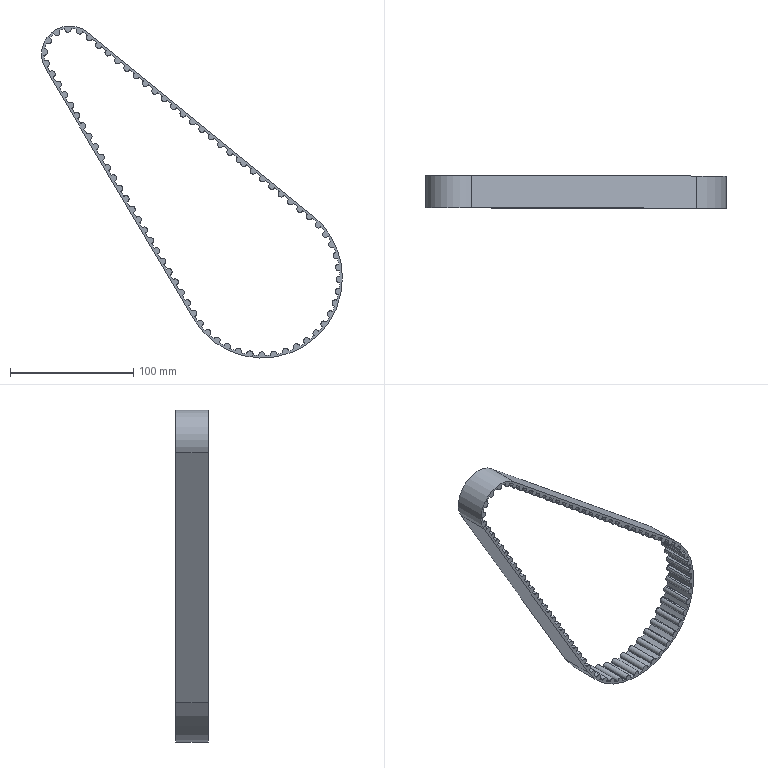Part | SolidWorks | features BaseBody 1 | 1 solid | 392 faces | box 243.977 x 26 x 269.227 mm | volume 64610 mm3 | plane 205 | cylinder 187 | commonest cylinder face diameters 5.2 x154 125.95 x23 41.98 x7 129.95 x2 45.98 x1